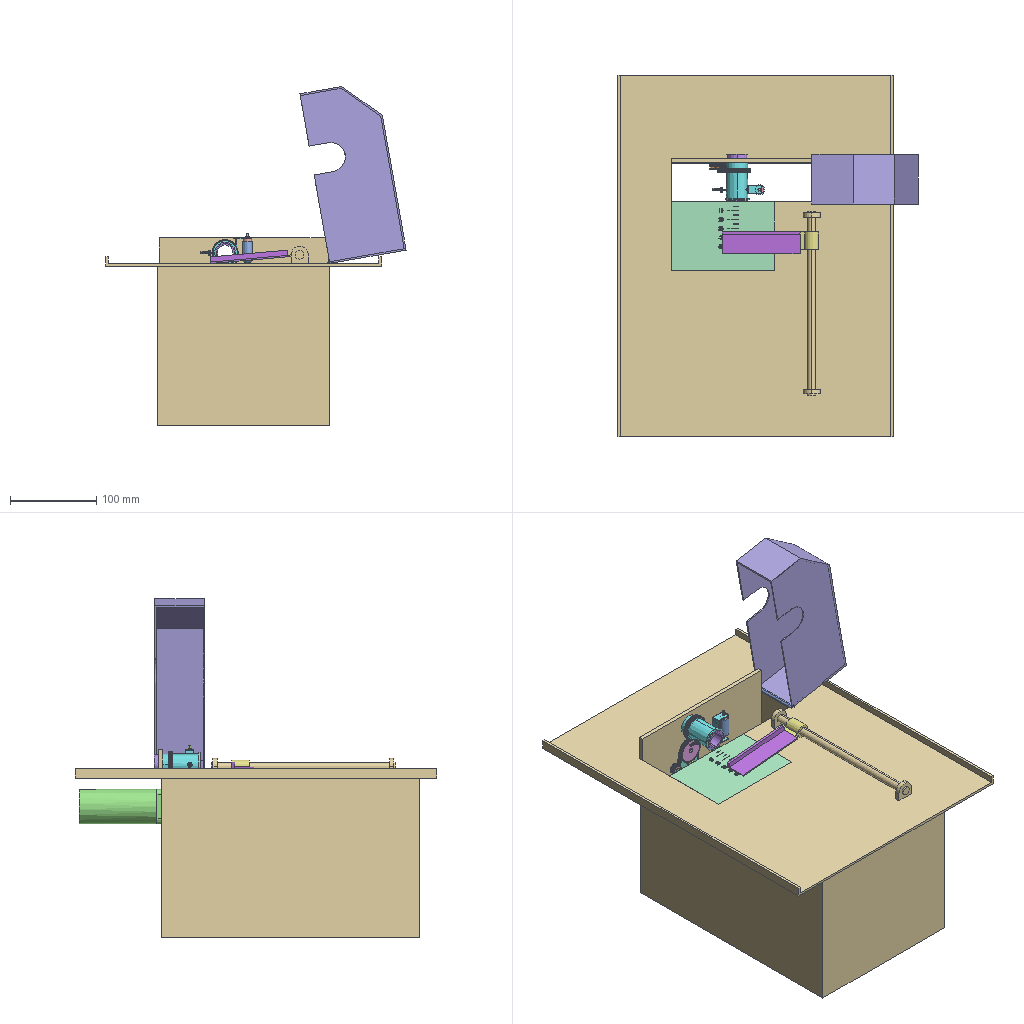Assembly | SolidWorks | 21 different items | 21 placed | box 349 x 420 x 393 mm
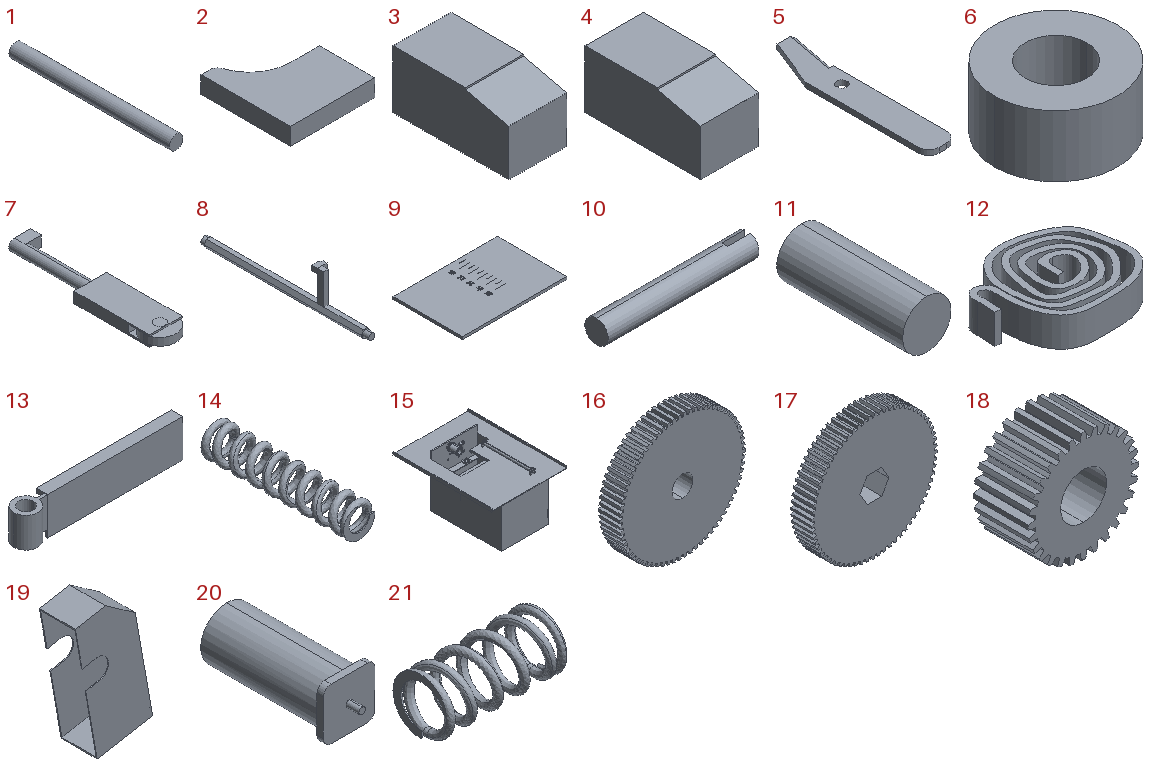Parts list (item | quantity | size | volume | features):
1 | x1 | 5 x 58.5 x 5 mm | 1149 mm3 | features BaseBody 1, ICE 1
2 | x1 | 9.85 x 10.458 x 2 mm | 150.551 mm3 | features Cut 2, Fillet 2, ICE 2, BaseBody 1
3 | x1 | 9 x 18 x 9 mm | 1396 mm3 | features BaseBody 1
4 | x1 | 9 x 18 x 9 mm | 1396 mm3 | features BaseBody 1
5 | x1 | 7.242 x 33.391 x 1 mm | 166.861 mm3 | features BaseBody 1, ICE 1
6 | x1 | 6 x 6 x 3 mm | 63.617 mm3 | features BaseBody 1
7 | x1 | 6.079 x 29.943 x 2 mm | 227.878 mm3 | features ICE 3, Cut 2, BaseBody 1
8 | x1 | 9.182 x 132 x 30 mm | 4582 mm3 | features ICE 6, Cut 3, BaseBody 1, Chamfer 1
9 | x1 | 120 x 80 x 3 mm | 28774 mm3 | features BaseBody 1
10 | x1 | 13 x 2 x 2 mm | 38.862 mm3 | features Extrusion 1, ICE 1
11 | x1 | 5 x 13 x 5 mm | 255.254 mm3 | features BaseBody 1
12 | x1 | 10.516 x 8.505 x 2.5 mm | 95.086 mm3 | features ICE 3, Fillet 2, Scale 1, Sweep 1
13 | x1 | 111.5 x 16 x 25 mm | 8047 mm3 | features ICE 3, Extrusion 1
14 | x1 | 2.498 x 11 x 2.497 mm | 11.802 mm3 | features BaseBody 1
15 | x1 | 320 x 420 x 222.634 mm | 1218802 mm3 | features ICE 27, Cut 8, Fillet 2, BaseBody 1, Chamfer 1, MirrorPattern 1, StudWizard 1
16 | x1 | 30 x 11 x 29.991 mm | 3758 mm3 | features BaseBody 1
17 | x1 | 29.999 x 5 x 29.999 mm | 3222 mm3 | features BaseBody 1
18 | x1 | 12 x 6 x 12 mm | 478.272 mm3 | features BaseBody 1
19 | x1 | 123.362 x 57.5 x 205.47 mm | 78596 mm3 | features ICE 3, BaseBody 1, Cut 1
20 | x1 | 40 x 105 x 40 mm | 121139 mm3 | features BaseBody 1
21 | x1 | 6 x 2.898 x 2.899 mm | 5.411 mm3 | features BaseBody 1
Mates (type | each side: item.copy, entity, surface, feature):
Concentric | 15.1 face cylinder Cut-Extrude1 | 10.1 face cylinder Boss-Extrude1
DistanceDim | 5.1 face plane Input 1 | 10.1 face plane Boss-Extrude1
Coincident | 15.1 face plane Input 1 | 12.1 face plane Sweep6
Parallel | 15.1 face plane Input 1 | 12.1 face plane Boss-Extrude2
Coincident | 10.1 face plane Cut-Extrude1 | 12.1 face plane Boss-Extrude2
Concentric | 15.1 face cylinder Boss-Extrude3 | 13.1 face cylinder Boss-Extrude1
Coincident | 15.1 face plane Input 1 | 13.1 edge
Coincident | 15.1 vertex | 9.1 vertex